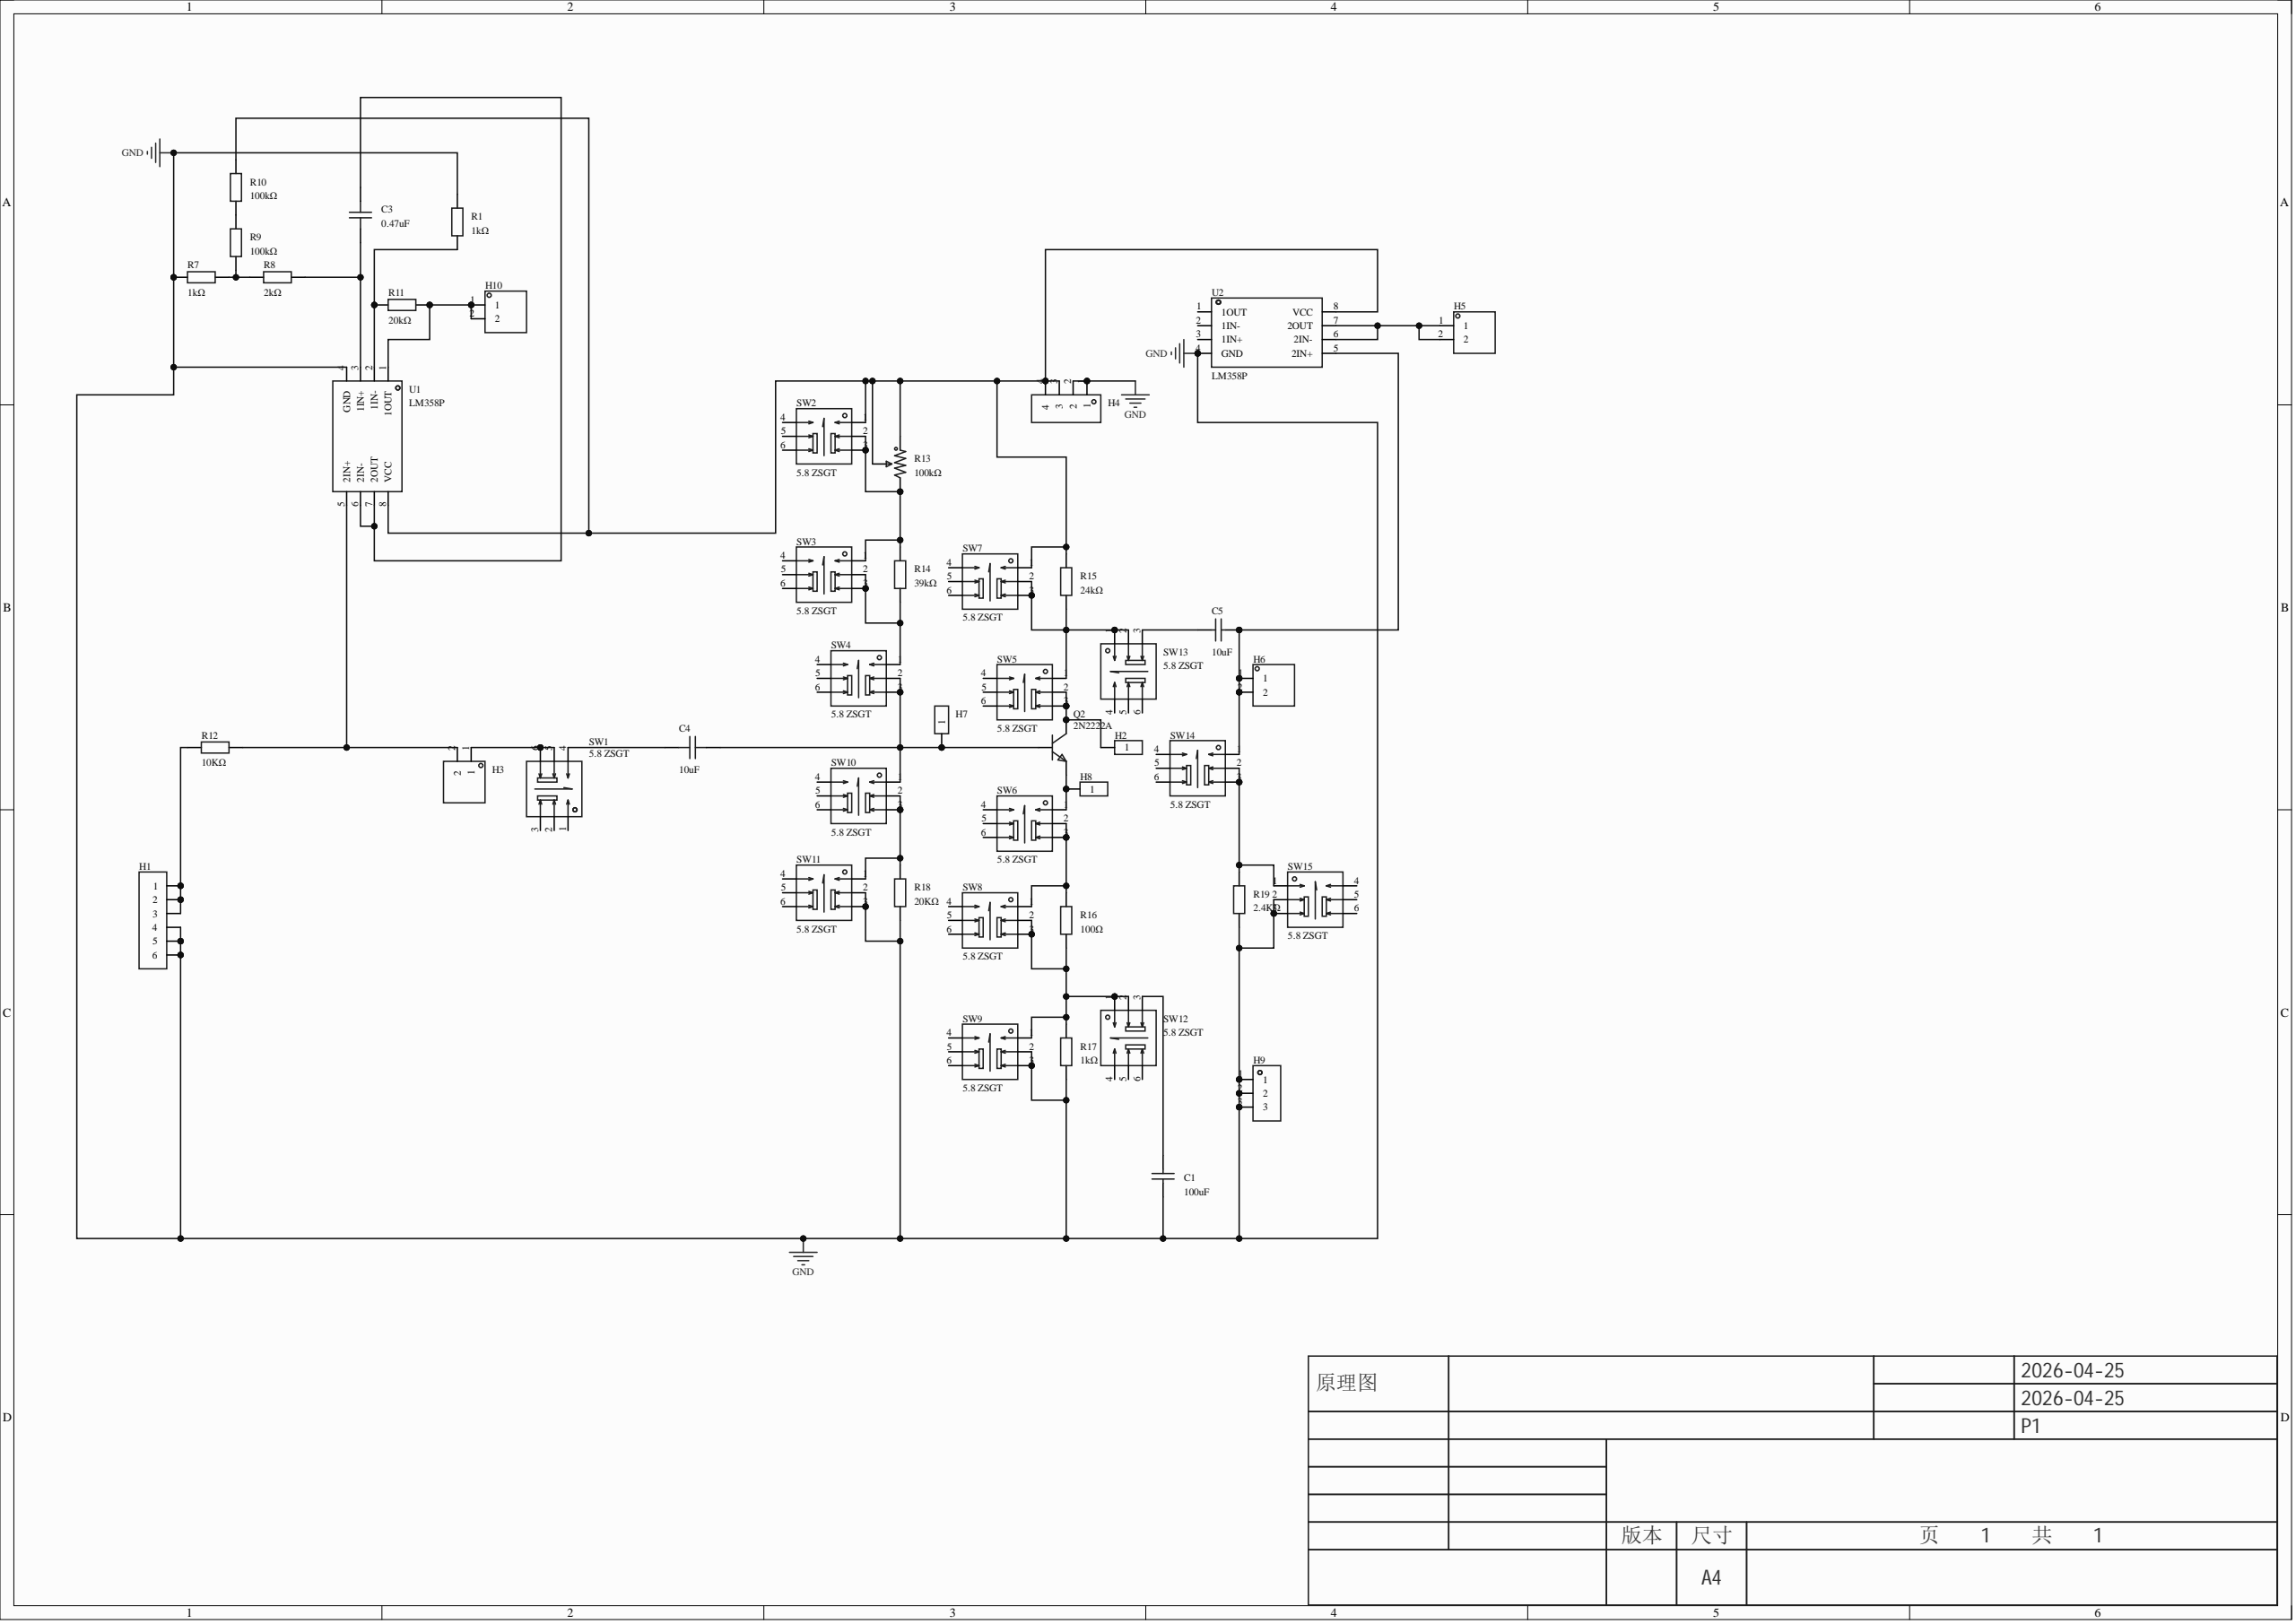Circuit board | Altium Designer | 46 parts | 26 nets
Bill of materials:
Comment,Description,Designator,Footprint,LibRef,Quantity
"100uF","容值:100uF;精度:±20%;额定电压:6.3V;温度系数:X5R;","C1","C0805","GRM21BR60J107ME15L","1"
"0.47uF","容值:10uF;精度:±10%;额定电压:10V;温度系数:X5R;","C3","C0603","CGA0603X5R106K100JT","1"
"10uF","容值:10uF;精度:±10%;额定电压:10V;温度系数:X5R;","C4","C0603","CGA0603X5R106K100JT","1"
"10uF","容值:100uF;精度:±20%;额定电压:6.3V;温度系数:X5R;","C5","C0805","GRM21BR60J107ME15L","1"
"","","H1","HDR-TH_6P-P2.54-V-M-1","HDR-M_2.54_1x6P","1"
"","","H2, H7, H8","HDR-TH_1P-V-M_XKB_X4611WV-01I-C28D40","HDR-M_2.54_1x1P","3"
"","","H3, H5, H6, H10","HDR-TH_2P-P2.54-V-M-1","HDR-M_2.54_1x2P","4"
"","","H4","HDR-TH_4P-P2.54-V-M","HDR-M_2.54_1x4P","1"
"","","H9","HDR-TH_3P-P2.54-V-M","HDR-M_2.54_1x3P","1"
"2N2222A","晶体管类型:NPN;集电极电流(Ic):600mA;集射极击穿电压(Vceo):40V;耗散功率(Pd):625mW;直流电流增益(hFE):40@500mA,10V;","Q2","TO-92-3_L4.9-W3.7-P1.27-L","2N2222A","1"
"1kΩ","","R1, R7, R17","R0603","0603WAF1001T5E, 0603WAF3902T5E","3"
"2kΩ","","R8","R0603","0603WAF1001T5E","1"
"100kΩ","","R9, R10","R0603","0603WAF1001T5E","2"
"20kΩ","","R11, R18","R0603","0603WAF1001T5E, 0603WAF3902T5E","2"
"10KΩ","","R12","R0603","RC0603FR-07100RL","1"
"100kΩ","","R13","RES-ADJ-SMD_JER33X-1-14","JER33X-1-15","1"
"39kΩ","","R14","R0603","0603WAF3902T5E","1"
"24kΩ","","R15","R0603","0603WAF3902T5E","1"
"100Ω","","R16","R0603","0603WAF3902T5E","1"
"2.4KΩ","","R19","R0603","0603WAF3902T5E","1"
"5.8 ZSGT","电路结构:双刀双掷;自锁/无锁:自锁;安装方式:直插;触点电流:110mA;额定电压:30V;带灯:不带;作用力:1.5N;工作寿命:10万次;","SW1, SW2, SW3, SW4, SW5, SW6, SW7, SW8, SW9, SW10, SW11, SW12, SW13, SW14, SW15","SW-TH_5.8ZSGT","5.8 ZSGT","15"
"LM358P","放大器数:双路;轨到轨:-;增益带宽积(GBP):-;输入失调电压(Vos):3mV;压摆率(SR):300V/ms;输入偏置电流(Ib):20nA;","U1, U2","DIP-8_L9.4-W6.4-P2.54-LS9.1-BL","LM358P","2"
Netlist (Protel format):
[
C1
C0805
100uF



]
[
C3
C0603
0.47uF



]
[
C4
C0603
10uF



]
[
C5
C0805
10uF



]
[
H1
HDR-TH_6P-P2.54-V-M-1




]
[
H2
HDR-TH_1P-V-M_XKB_X4611WV-01I-C28D40




]
[
H3
HDR-TH_2P-P2.54-V-M-1




]
[
H4
HDR-TH_4P-P2.54-V-M




]
[
H5
HDR-TH_2P-P2.54-V-M-1




]
[
H6
HDR-TH_2P-P2.54-V-M-1




]
[
H7
HDR-TH_1P-V-M_XKB_X4611WV-01I-C28D40




]
[
H8
HDR-TH_1P-V-M_XKB_X4611WV-01I-C28D40




]
[
H9
HDR-TH_3P-P2.54-V-M




]
[
H10
HDR-TH_2P-P2.54-V-M-1




]
[
Q2
TO-92-3_L4.9-W3.7-P1.27-L
2N2222A



]
[
R1
R0603
1kΩ



]
[
R7
R0603
1kΩ



]
[
R8
R0603
2kΩ



]
[
R9
R0603
100kΩ



]
[
R10
R0603
100kΩ



]
[
R11
R0603
20kΩ



]
[
R12
R0603
10KΩ



]
[
R13
RES-ADJ-SMD_JER33X-1-14
100kΩ



]
[
R14
R0603
39kΩ



]
[
R15
R0603
24kΩ



]
[
R16
R0603
100Ω



]
[
R17
R0603
1kΩ



]
[
R18
R0603
20KΩ



]
[
R19
R0603
2.4KΩ



]
[
SW1
SW-TH_5.8ZSGT
5.8 ZSGT



]
[
SW2
SW-TH_5.8ZSGT
5.8 ZSGT



]
[
SW3
SW-TH_5.8ZSGT
5.8 ZSGT



]
[
SW4
SW-TH_5.8ZSGT
5.8 ZSGT



]
[
SW5
SW-TH_5.8ZSGT
5.8 ZSGT



]
[
SW6
SW-TH_5.8ZSGT
5.8 ZSGT



]
[
SW7
SW-TH_5.8ZSGT
5.8 ZSGT



]
[
SW8
SW-TH_5.8ZSGT
5.8 ZSGT



]
[
SW9
SW-TH_5.8ZSGT
5.8 ZSGT



]
[
SW10
SW-TH_5.8ZSGT
5.8 ZSGT



]
[
SW11
SW-TH_5.8ZSGT
5.8 ZSGT



]
[
SW12
SW-TH_5.8ZSGT
5.8 ZSGT



]
[
SW13
SW-TH_5.8ZSGT
5.8 ZSGT



]
[
SW14
SW-TH_5.8ZSGT
5.8 ZSGT



]
[
SW15
SW-TH_5.8ZSGT
5.8 ZSGT



]
[
U1
DIP-8_L9.4-W6.4-P2.54-LS9.1-BL
LM358P



]
[
U2
DIP-8_L9.4-W6.4-P2.54-LS9.1-BL
LM358P



]
(
NetR19_2
R19-2
SW14-2
SW14-3
SW15-1
)
(
NetR18_2
R18-2
SW10-2
SW10-3
SW11-1
)
(
NetR16_2
R16-2
SW6-2
SW6-3
SW8-1
)
(
NetR16_1
R16-1
R17-2
SW8-2
SW8-3
SW9-1
SW12-1
SW12-2
)
(
NetR15_1
R15-1
SW5-1
SW7-2
SW7-3
SW13-1
SW13-2
)
(
NetR14_1
R14-1
SW3-2
SW3-3
SW4-1
)
(
NetR13_3
R13-3
R14-2
SW2-2
SW2-3
SW3-1
)
(
NetR9_2
R9-2
R10-1
)
(
NetR7_2
R7-2
R8-1
R9-1
)
(
NetR1_1
R1-1
R11-1
U1-2
)
(
NetH10_1
H10-1
H10-2
R11-2
U1-1
)
(
NetH8_1
H8-1
Q2-1
SW6-1
)
(
NetH5_1
H5-1
H5-2
U2-6
U2-7
)
(
NetH4_3
H4-3
H4-4
R10-2
R13-1
R13-2
R15-2
SW2-1
SW7-1
U1-8
U2-8
)
(
NetH3_2
H3-2
R12-2
U1-5
)
(
NetH3_1
H3-1
SW1-5
SW1-6
)
(
NetH2_1
H2-1
Q2-3
SW5-2
SW5-3
)
(
NetH1_1
H1-1
H1-2
H1-3
R12-1
)
(
NetC5_2
C5-2
SW13-3
)
(
NetC5_1
C5-1
H6-1
H6-2
SW14-1
U2-5
)
(
NetC4_2
C4-2
H7-1
Q2-2
SW4-2
SW4-3
SW10-1
)
(
NetC4_1
C4-1
SW1-4
)
(
NetC3_2
C3-2
U1-6
U1-7
)
(
NetC3_1
C3-1
R8-2
U1-3
)
(
NetC1_2
C1-2
SW12-3
)
(
GND
C1-1
H1-4
H1-5
H1-6
H4-1
H4-2
H9-1
H9-2
H9-3
R1-2
R7-1
R17-1
R18-1
R19-1
SW9-2
SW9-3
SW11-2
SW11-3
SW15-2
SW15-3
U1-4
U2-4
)